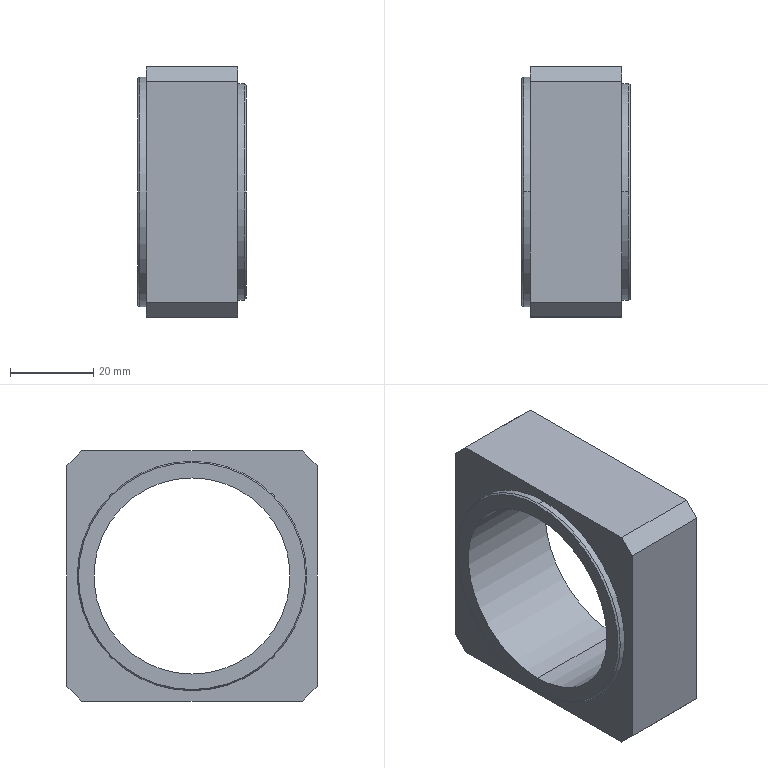Part | STEP file | _Kupplungsgehaeuse-SBG - PAS42 B | 1 solid | 22 faces | box 26 x 60 x 60 mm | volume 42515 mm3 | plane 12 | cylinder 6 | cone 4 | commonest cylinder face diameters 47 x2 52 x2 55 x2
STEP:
#1=CARTESIAN_POINT('',(26.,0.,-23.5));
#2=VERTEX_POINT('',#1);
#3=CARTESIAN_POINT('',(26.,0.,23.5));
#4=VERTEX_POINT('',#3);
#5=CARTESIAN_POINT('',(26.,0.,0.));
#6=DIRECTION('',(-1.,0.,0.));
#7=DIRECTION('',(0.,0.,1.));
#8=AXIS2_PLACEMENT_3D('',#5,#6,#7);
#9=CIRCLE('',#8,23.5);
#10=EDGE_CURVE('',#2,#4,#9,.T.);
#11=ORIENTED_EDGE('',*,*,#10,.F.);
#12=CARTESIAN_POINT('',(0.,0.,-23.5));
#13=VERTEX_POINT('',#12);
#14=CARTESIAN_POINT('',(26.,0.,-23.5));
#15=DIRECTION('',(-1.,0.,0.));
#16=VECTOR('',#15,1000.);
#17=LINE('',#14,#16);
#18=EDGE_CURVE('',#2,#13,#17,.T.);
#19=ORIENTED_EDGE('',*,*,#18,.T.);
#20=CARTESIAN_POINT('',(0.,0.,23.5));
#21=VERTEX_POINT('',#20);
#22=CARTESIAN_POINT('',(0.,0.,0.));
#23=DIRECTION('',(1.,0.,0.));
#24=DIRECTION('',(0.,0.,1.));
#25=AXIS2_PLACEMENT_3D('',#22,#23,#24);
#26=CIRCLE('',#25,23.5);
#27=EDGE_CURVE('',#21,#13,#26,.T.);
#28=ORIENTED_EDGE('',*,*,#27,.F.);
#29=CARTESIAN_POINT('',(26.,0.,23.5));
#30=DIRECTION('',(-1.,0.,0.));
#31=VECTOR('',#30,1000.);
#32=LINE('',#29,#31);
#33=EDGE_CURVE('',#4,#21,#32,.T.);
#34=ORIENTED_EDGE('',*,*,#33,.F.);
#35=EDGE_LOOP('',(#11,#19,#28,#34));
#36=FACE_OUTER_BOUND('',#35,.T.);
#37=CARTESIAN_POINT('',(26.,0.,0.));
#38=DIRECTION('',(-1.,0.,0.));
#39=DIRECTION('',(0.,0.,1.));
#40=AXIS2_PLACEMENT_3D('',#37,#38,#39);
#41=CYLINDRICAL_SURFACE('',#40,23.5);
#42=ADVANCED_FACE('',(#36),#41,.F.);
#43=CARTESIAN_POINT('',(0.,-27.211,0.));
#44=VERTEX_POINT('',#43);
#45=CARTESIAN_POINT('',(0.,27.211,0.));
#46=VERTEX_POINT('',#45);
#47=CARTESIAN_POINT('',(0.,0.,0.));
#48=DIRECTION('',(-1.,0.,0.));
#49=DIRECTION('',(0.,1.,0.));
#50=AXIS2_PLACEMENT_3D('',#47,#48,#49);
#51=CIRCLE('',#50,27.211);
#52=EDGE_CURVE('',#44,#46,#51,.T.);
#53=ORIENTED_EDGE('',*,*,#52,.F.);
#54=CARTESIAN_POINT('',(0.5,-27.5,0.));
#55=VERTEX_POINT('',#54);
#56=CARTESIAN_POINT('',(0.5,-27.5,0.));
#57=DIRECTION('',(0.866,-0.5,0.));
#58=VECTOR('',#57,1000.);
#59=LINE('',#56,#58);
#60=EDGE_CURVE('',#44,#55,#59,.T.);
#61=ORIENTED_EDGE('',*,*,#60,.T.);
#62=CARTESIAN_POINT('',(0.5,0.,27.5));
#63=VERTEX_POINT('',#62);
#64=CARTESIAN_POINT('',(0.5,0.,0.));
#65=DIRECTION('',(-1.,0.,0.));
#66=DIRECTION('',(0.,0.,-1.));
#67=AXIS2_PLACEMENT_3D('',#64,#65,#66);
#68=CIRCLE('',#67,27.5);
#69=EDGE_CURVE('',#55,#63,#68,.T.);
#70=ORIENTED_EDGE('',*,*,#69,.T.);
#71=CARTESIAN_POINT('',(0.5,27.5,0.));
#72=VERTEX_POINT('',#71);
#73=CARTESIAN_POINT('',(0.5,0.,0.));
#74=DIRECTION('',(-1.,0.,0.));
#75=DIRECTION('',(0.,0.,-1.));
#76=AXIS2_PLACEMENT_3D('',#73,#74,#75);
#77=CIRCLE('',#76,27.5);
#78=EDGE_CURVE('',#63,#72,#77,.T.);
#79=ORIENTED_EDGE('',*,*,#78,.T.);
#80=CARTESIAN_POINT('',(0.5,27.5,0.));
#81=DIRECTION('',(0.866,0.5,0.));
#82=VECTOR('',#81,1000.);
#83=LINE('',#80,#82);
#84=EDGE_CURVE('',#46,#72,#83,.T.);
#85=ORIENTED_EDGE('',*,*,#84,.F.);
#86=EDGE_LOOP('',(#53,#61,#70,#79,#85));
#87=FACE_OUTER_BOUND('',#86,.T.);
#88=CARTESIAN_POINT('',(0.5,0.,0.));
#89=DIRECTION('',(1.,0.,0.));
#90=DIRECTION('',(0.,1.,0.));
#91=AXIS2_PLACEMENT_3D('',#88,#89,#90);
#92=CONICAL_SURFACE('',#91,27.5,0.5236);
#93=ADVANCED_FACE('',(#87),#92,.T.);
#94=CARTESIAN_POINT('',(26.,25.711,0.));
#95=VERTEX_POINT('',#94);
#96=CARTESIAN_POINT('',(26.,-25.711,0.));
#97=VERTEX_POINT('',#96);
#98=CARTESIAN_POINT('',(26.,0.,0.));
#99=DIRECTION('',(1.,0.,0.));
#100=DIRECTION('',(0.,-1.,0.));
#101=AXIS2_PLACEMENT_3D('',#98,#99,#100);
#102=CIRCLE('',#101,25.711);
#103=EDGE_CURVE('',#95,#97,#102,.T.);
#104=ORIENTED_EDGE('',*,*,#103,.F.);
#105=CARTESIAN_POINT('',(25.5,26.,0.));
#106=VERTEX_POINT('',#105);
#107=CARTESIAN_POINT('',(25.5,26.,0.));
#108=DIRECTION('',(-0.866,0.5,0.));
#109=VECTOR('',#108,1000.);
#110=LINE('',#107,#109);
#111=EDGE_CURVE('',#95,#106,#110,.T.);
#112=ORIENTED_EDGE('',*,*,#111,.T.);
#113=CARTESIAN_POINT('',(25.5,0.,26.));
#114=VERTEX_POINT('',#113);
#115=CARTESIAN_POINT('',(25.5,0.,0.));
#116=DIRECTION('',(1.,0.,0.));
#117=DIRECTION('',(0.,0.,1.));
#118=AXIS2_PLACEMENT_3D('',#115,#116,#117);
#119=CIRCLE('',#118,26.);
#120=EDGE_CURVE('',#106,#114,#119,.T.);
#121=ORIENTED_EDGE('',*,*,#120,.T.);
#122=CARTESIAN_POINT('',(25.5,-26.,0.));
#123=VERTEX_POINT('',#122);
#124=CARTESIAN_POINT('',(25.5,0.,0.));
#125=DIRECTION('',(1.,0.,0.));
#126=DIRECTION('',(0.,0.,1.));
#127=AXIS2_PLACEMENT_3D('',#124,#125,#126);
#128=CIRCLE('',#127,26.);
#129=EDGE_CURVE('',#114,#123,#128,.T.);
#130=ORIENTED_EDGE('',*,*,#129,.T.);
#131=CARTESIAN_POINT('',(25.5,-26.,0.));
#132=DIRECTION('',(-0.866,-0.5,0.));
#133=VECTOR('',#132,1000.);
#134=LINE('',#131,#133);
#135=EDGE_CURVE('',#97,#123,#134,.T.);
#136=ORIENTED_EDGE('',*,*,#135,.F.);
#137=EDGE_LOOP('',(#104,#112,#121,#130,#136));
#138=FACE_OUTER_BOUND('',#137,.T.);
#139=CARTESIAN_POINT('',(25.5,0.,0.));
#140=DIRECTION('',(-1.,0.,0.));
#141=DIRECTION('',(0.,-1.,0.));
#142=AXIS2_PLACEMENT_3D('',#139,#140,#141);
#143=CONICAL_SURFACE('',#142,26.,0.5236);
#144=ADVANCED_FACE('',(#138),#143,.T.);
#145=CARTESIAN_POINT('',(2.,0.,27.5));
#146=VERTEX_POINT('',#145);
#147=CARTESIAN_POINT('',(2.,0.,-27.5));
#148=VERTEX_POINT('',#147);
#149=CARTESIAN_POINT('',(2.,0.,0.));
#150=DIRECTION('',(-1.,0.,0.));
#151=DIRECTION('',(0.,0.,1.));
#152=AXIS2_PLACEMENT_3D('',#149,#150,#151);
#153=CIRCLE('',#152,27.5);
#154=EDGE_CURVE('',#146,#148,#153,.T.);
#155=ORIENTED_EDGE('',*,*,#154,.T.);
#156=CARTESIAN_POINT('',(0.5,0.,-27.5));
#157=VERTEX_POINT('',#156);
#158=CARTESIAN_POINT('',(26.,0.,-27.5));
#159=DIRECTION('',(-1.,0.,0.));
#160=VECTOR('',#159,1000.);
#161=LINE('',#158,#160);
#162=EDGE_CURVE('',#148,#157,#161,.T.);
#163=ORIENTED_EDGE('',*,*,#162,.T.);
#164=CARTESIAN_POINT('',(0.5,0.,0.));
#165=DIRECTION('',(-1.,0.,0.));
#166=DIRECTION('',(0.,0.,-1.));
#167=AXIS2_PLACEMENT_3D('',#164,#165,#166);
#168=CIRCLE('',#167,27.5);
#169=EDGE_CURVE('',#72,#157,#168,.T.);
#170=ORIENTED_EDGE('',*,*,#169,.F.);
#171=ORIENTED_EDGE('',*,*,#78,.F.);
#172=CARTESIAN_POINT('',(26.,0.,27.5));
#173=DIRECTION('',(-1.,0.,0.));
#174=VECTOR('',#173,1000.);
#175=LINE('',#172,#174);
#176=EDGE_CURVE('',#146,#63,#175,.T.);
#177=ORIENTED_EDGE('',*,*,#176,.F.);
#178=EDGE_LOOP('',(#155,#163,#170,#171,#177));
#179=FACE_OUTER_BOUND('',#178,.T.);
#180=CARTESIAN_POINT('',(26.,0.,0.));
#181=DIRECTION('',(-1.,0.,0.));
#182=DIRECTION('',(0.,0.,1.));
#183=AXIS2_PLACEMENT_3D('',#180,#181,#182);
#184=CYLINDRICAL_SURFACE('',#183,27.5);
#185=ADVANCED_FACE('',(#179),#184,.T.);
#186=CARTESIAN_POINT('',(25.5,0.,-26.));
#187=VERTEX_POINT('',#186);
#188=CARTESIAN_POINT('',(25.5,0.,0.));
#189=DIRECTION('',(1.,0.,0.));
#190=DIRECTION('',(0.,0.,1.));
#191=AXIS2_PLACEMENT_3D('',#188,#189,#190);
#192=CIRCLE('',#191,26.);
#193=EDGE_CURVE('',#187,#106,#192,.T.);
#194=ORIENTED_EDGE('',*,*,#193,.F.);
#195=CARTESIAN_POINT('',(24.,0.,-26.));
#196=VERTEX_POINT('',#195);
#197=CARTESIAN_POINT('',(26.,0.,-26.));
#198=DIRECTION('',(-1.,0.,0.));
#199=VECTOR('',#198,1000.);
#200=LINE('',#197,#199);
#201=EDGE_CURVE('',#187,#196,#200,.T.);
#202=ORIENTED_EDGE('',*,*,#201,.T.);
#203=CARTESIAN_POINT('',(24.,0.,26.));
#204=VERTEX_POINT('',#203);
#205=CARTESIAN_POINT('',(24.,0.,0.));
#206=DIRECTION('',(1.,0.,0.));
#207=DIRECTION('',(0.,0.,1.));
#208=AXIS2_PLACEMENT_3D('',#205,#206,#207);
#209=CIRCLE('',#208,26.);
#210=EDGE_CURVE('',#196,#204,#209,.T.);
#211=ORIENTED_EDGE('',*,*,#210,.T.);
#212=CARTESIAN_POINT('',(26.,0.,26.));
#213=DIRECTION('',(-1.,0.,0.));
#214=VECTOR('',#213,1000.);
#215=LINE('',#212,#214);
#216=EDGE_CURVE('',#114,#204,#215,.T.);
#217=ORIENTED_EDGE('',*,*,#216,.F.);
#218=ORIENTED_EDGE('',*,*,#120,.F.);
#219=EDGE_LOOP('',(#194,#202,#211,#217,#218));
#220=FACE_OUTER_BOUND('',#219,.T.);
#221=CARTESIAN_POINT('',(26.,0.,0.));
#222=DIRECTION('',(-1.,0.,0.));
#223=DIRECTION('',(0.,0.,1.));
#224=AXIS2_PLACEMENT_3D('',#221,#222,#223);
#225=CYLINDRICAL_SURFACE('',#224,26.);
#226=ADVANCED_FACE('',(#220),#225,.T.);
#227=ORIENTED_EDGE('',*,*,#18,.F.);
#228=CARTESIAN_POINT('',(26.,0.,0.));
#229=DIRECTION('',(-1.,0.,0.));
#230=DIRECTION('',(0.,0.,1.));
#231=AXIS2_PLACEMENT_3D('',#228,#229,#230);
#232=CIRCLE('',#231,23.5);
#233=EDGE_CURVE('',#4,#2,#232,.T.);
#234=ORIENTED_EDGE('',*,*,#233,.F.);
#235=ORIENTED_EDGE('',*,*,#33,.T.);
#236=CARTESIAN_POINT('',(0.,0.,0.));
#237=DIRECTION('',(1.,0.,0.));
#238=DIRECTION('',(0.,0.,1.));
#239=AXIS2_PLACEMENT_3D('',#236,#237,#238);
#240=CIRCLE('',#239,23.5);
#241=EDGE_CURVE('',#13,#21,#240,.T.);
#242=ORIENTED_EDGE('',*,*,#241,.F.);
#243=EDGE_LOOP('',(#227,#234,#235,#242));
#244=FACE_OUTER_BOUND('',#243,.T.);
#245=CARTESIAN_POINT('',(26.,0.,0.));
#246=DIRECTION('',(-1.,0.,0.));
#247=DIRECTION('',(0.,0.,1.));
#248=AXIS2_PLACEMENT_3D('',#245,#246,#247);
#249=CYLINDRICAL_SURFACE('',#248,23.5);
#250=ADVANCED_FACE('',(#244),#249,.F.);
#251=CARTESIAN_POINT('',(0.,0.,0.));
#252=DIRECTION('',(-1.,0.,0.));
#253=DIRECTION('',(0.,1.,0.));
#254=AXIS2_PLACEMENT_3D('',#251,#252,#253);
#255=CIRCLE('',#254,27.211);
#256=EDGE_CURVE('',#46,#44,#255,.T.);
#257=ORIENTED_EDGE('',*,*,#256,.T.);
#258=ORIENTED_EDGE('',*,*,#52,.T.);
#259=EDGE_LOOP('',(#257,#258));
#260=FACE_OUTER_BOUND('',#259,.T.);
#261=ORIENTED_EDGE('',*,*,#27,.T.);
#262=ORIENTED_EDGE('',*,*,#241,.T.);
#263=EDGE_LOOP('',(#261,#262));
#264=FACE_BOUND('',#263,.T.);
#265=CARTESIAN_POINT('',(0.,27.211,0.));
#266=DIRECTION('',(-1.,0.,0.));
#267=DIRECTION('',(0.,0.,1.));
#268=AXIS2_PLACEMENT_3D('',#265,#266,#267);
#269=PLANE('',#268);
#270=ADVANCED_FACE('',(#260,#264),#269,.T.);
#271=ORIENTED_EDGE('',*,*,#233,.T.);
#272=ORIENTED_EDGE('',*,*,#10,.T.);
#273=EDGE_LOOP('',(#271,#272));
#274=FACE_BOUND('',#273,.T.);
#275=CARTESIAN_POINT('',(26.,0.,0.));
#276=DIRECTION('',(1.,0.,0.));
#277=DIRECTION('',(0.,-1.,0.));
#278=AXIS2_PLACEMENT_3D('',#275,#276,#277);
#279=CIRCLE('',#278,25.711);
#280=EDGE_CURVE('',#97,#95,#279,.T.);
#281=ORIENTED_EDGE('',*,*,#280,.T.);
#282=ORIENTED_EDGE('',*,*,#103,.T.);
#283=EDGE_LOOP('',(#281,#282));
#284=FACE_OUTER_BOUND('',#283,.T.);
#285=CARTESIAN_POINT('',(26.,23.5,0.));
#286=DIRECTION('',(1.,0.,0.));
#287=DIRECTION('',(0.,0.,-1.));
#288=AXIS2_PLACEMENT_3D('',#285,#286,#287);
#289=PLANE('',#288);
#290=ADVANCED_FACE('',(#274,#284),#289,.T.);
#291=ORIENTED_EDGE('',*,*,#60,.F.);
#292=ORIENTED_EDGE('',*,*,#256,.F.);
#293=ORIENTED_EDGE('',*,*,#84,.T.);
#294=ORIENTED_EDGE('',*,*,#169,.T.);
#295=CARTESIAN_POINT('',(0.5,0.,0.));
#296=DIRECTION('',(-1.,0.,0.));
#297=DIRECTION('',(0.,0.,-1.));
#298=AXIS2_PLACEMENT_3D('',#295,#296,#297);
#299=CIRCLE('',#298,27.5);
#300=EDGE_CURVE('',#157,#55,#299,.T.);
#301=ORIENTED_EDGE('',*,*,#300,.T.);
#302=EDGE_LOOP('',(#291,#292,#293,#294,#301));
#303=FACE_OUTER_BOUND('',#302,.T.);
#304=CARTESIAN_POINT('',(0.5,0.,0.));
#305=DIRECTION('',(1.,0.,0.));
#306=DIRECTION('',(0.,1.,0.));
#307=AXIS2_PLACEMENT_3D('',#304,#305,#306);
#308=CONICAL_SURFACE('',#307,27.5,0.5236);
#309=ADVANCED_FACE('',(#303),#308,.T.);
#310=ORIENTED_EDGE('',*,*,#111,.F.);
#311=ORIENTED_EDGE('',*,*,#280,.F.);
#312=ORIENTED_EDGE('',*,*,#135,.T.);
#313=CARTESIAN_POINT('',(25.5,0.,0.));
#314=DIRECTION('',(1.,0.,0.));
#315=DIRECTION('',(0.,0.,1.));
#316=AXIS2_PLACEMENT_3D('',#313,#314,#315);
#317=CIRCLE('',#316,26.);
#318=EDGE_CURVE('',#123,#187,#317,.T.);
#319=ORIENTED_EDGE('',*,*,#318,.T.);
#320=ORIENTED_EDGE('',*,*,#193,.T.);
#321=EDGE_LOOP('',(#310,#311,#312,#319,#320));
#322=FACE_OUTER_BOUND('',#321,.T.);
#323=CARTESIAN_POINT('',(25.5,0.,0.));
#324=DIRECTION('',(-1.,0.,0.));
#325=DIRECTION('',(0.,-1.,0.));
#326=AXIS2_PLACEMENT_3D('',#323,#324,#325);
#327=CONICAL_SURFACE('',#326,26.,0.5236);
#328=ADVANCED_FACE('',(#322),#327,.T.);
#329=ORIENTED_EDGE('',*,*,#162,.F.);
#330=CARTESIAN_POINT('',(2.,0.,0.));
#331=DIRECTION('',(-1.,0.,0.));
#332=DIRECTION('',(0.,0.,1.));
#333=AXIS2_PLACEMENT_3D('',#330,#331,#332);
#334=CIRCLE('',#333,27.5);
#335=EDGE_CURVE('',#148,#146,#334,.T.);
#336=ORIENTED_EDGE('',*,*,#335,.T.);
#337=ORIENTED_EDGE('',*,*,#176,.T.);
#338=ORIENTED_EDGE('',*,*,#69,.F.);
#339=ORIENTED_EDGE('',*,*,#300,.F.);
#340=EDGE_LOOP('',(#329,#336,#337,#338,#339));
#341=FACE_OUTER_BOUND('',#340,.T.);
#342=CARTESIAN_POINT('',(26.,0.,0.));
#343=DIRECTION('',(-1.,0.,0.));
#344=DIRECTION('',(0.,0.,1.));
#345=AXIS2_PLACEMENT_3D('',#342,#343,#344);
#346=CYLINDRICAL_SURFACE('',#345,27.5);
#347=ADVANCED_FACE('',(#341),#346,.T.);
#348=ORIENTED_EDGE('',*,*,#201,.F.);
#349=ORIENTED_EDGE('',*,*,#318,.F.);
#350=ORIENTED_EDGE('',*,*,#129,.F.);
#351=ORIENTED_EDGE('',*,*,#216,.T.);
#352=CARTESIAN_POINT('',(24.,0.,0.));
#353=DIRECTION('',(1.,0.,0.));
#354=DIRECTION('',(0.,0.,1.));
#355=AXIS2_PLACEMENT_3D('',#352,#353,#354);
#356=CIRCLE('',#355,26.);
#357=EDGE_CURVE('',#204,#196,#356,.T.);
#358=ORIENTED_EDGE('',*,*,#357,.T.);
#359=EDGE_LOOP('',(#348,#349,#350,#351,#358));
#360=FACE_OUTER_BOUND('',#359,.T.);
#361=CARTESIAN_POINT('',(26.,0.,0.));
#362=DIRECTION('',(-1.,0.,0.));
#363=DIRECTION('',(0.,0.,1.));
#364=AXIS2_PLACEMENT_3D('',#361,#362,#363);
#365=CYLINDRICAL_SURFACE('',#364,26.);
#366=ADVANCED_FACE('',(#360),#365,.T.);
#367=CARTESIAN_POINT('',(2.,30.,26.46));
#368=VERTEX_POINT('',#367);
#369=CARTESIAN_POINT('',(2.,26.46,30.));
#370=VERTEX_POINT('',#369);
#371=CARTESIAN_POINT('',(2.,30.,26.46));
#372=DIRECTION('',(0.,-0.7071,0.7071));
#373=VECTOR('',#372,1000.);
#374=LINE('',#371,#373);
#375=EDGE_CURVE('',#368,#370,#374,.T.);
#376=ORIENTED_EDGE('',*,*,#375,.F.);
#377=CARTESIAN_POINT('',(2.,30.,-26.46));
#378=VERTEX_POINT('',#377);
#379=CARTESIAN_POINT('',(2.,30.,0.));
#380=DIRECTION('',(0.,0.,1.));
#381=VECTOR('',#380,1000.);
#382=LINE('',#379,#381);
#383=EDGE_CURVE('',#378,#368,#382,.T.);
#384=ORIENTED_EDGE('',*,*,#383,.F.);
#385=CARTESIAN_POINT('',(2.,26.46,-30.));
#386=VERTEX_POINT('',#385);
#387=CARTESIAN_POINT('',(2.,26.46,-30.));
#388=DIRECTION('',(0.,0.7071,0.7071));
#389=VECTOR('',#388,1000.);
#390=LINE('',#387,#389);
#391=EDGE_CURVE('',#386,#378,#390,.T.);
#392=ORIENTED_EDGE('',*,*,#391,.F.);
#393=CARTESIAN_POINT('',(2.,-26.46,-30.));
#394=VERTEX_POINT('',#393);
#395=CARTESIAN_POINT('',(2.,0.,-30.));
#396=DIRECTION('',(0.,1.,0.));
#397=VECTOR('',#396,1000.);
#398=LINE('',#395,#397);
#399=EDGE_CURVE('',#394,#386,#398,.T.);
#400=ORIENTED_EDGE('',*,*,#399,.F.);
#401=CARTESIAN_POINT('',(2.,-30.,-26.46));
#402=VERTEX_POINT('',#401);
#403=CARTESIAN_POINT('',(2.,-30.,-26.46));
#404=DIRECTION('',(0.,0.7071,-0.7071));
#405=VECTOR('',#404,1000.);
#406=LINE('',#403,#405);
#407=EDGE_CURVE('',#402,#394,#406,.T.);
#408=ORIENTED_EDGE('',*,*,#407,.F.);
#409=CARTESIAN_POINT('',(2.,-30.,26.46));
#410=VERTEX_POINT('',#409);
#411=CARTESIAN_POINT('',(2.,-30.,0.));
#412=DIRECTION('',(0.,0.,-1.));
#413=VECTOR('',#412,1000.);
#414=LINE('',#411,#413);
#415=EDGE_CURVE('',#410,#402,#414,.T.);
#416=ORIENTED_EDGE('',*,*,#415,.F.);
#417=CARTESIAN_POINT('',(2.,-26.46,30.));
#418=VERTEX_POINT('',#417);
#419=CARTESIAN_POINT('',(2.,-26.46,30.));
#420=DIRECTION('',(0.,-0.7071,-0.7071));
#421=VECTOR('',#420,1000.);
#422=LINE('',#419,#421);
#423=EDGE_CURVE('',#418,#410,#422,.T.);
#424=ORIENTED_EDGE('',*,*,#423,.F.);
#425=CARTESIAN_POINT('',(2.,0.,30.));
#426=DIRECTION('',(0.,-1.,0.));
#427=VECTOR('',#426,1000.);
#428=LINE('',#425,#427);
#429=EDGE_CURVE('',#370,#418,#428,.T.);
#430=ORIENTED_EDGE('',*,*,#429,.F.);
#431=EDGE_LOOP('',(#376,#384,#392,#400,#408,#416,#424,#430));
#432=FACE_OUTER_BOUND('',#431,.T.);
#433=ORIENTED_EDGE('',*,*,#154,.F.);
#434=ORIENTED_EDGE('',*,*,#335,.F.);
#435=EDGE_LOOP('',(#433,#434));
#436=FACE_BOUND('',#435,.T.);
#437=CARTESIAN_POINT('',(2.,0.,0.));
#438=DIRECTION('',(1.,0.,0.));
#439=DIRECTION('',(0.,0.,-1.));
#440=AXIS2_PLACEMENT_3D('',#437,#438,#439);
#441=PLANE('',#440);
#442=ADVANCED_FACE('',(#432,#436),#441,.F.);
#443=CARTESIAN_POINT('',(24.,30.,-26.46));
#444=VERTEX_POINT('',#443);
#445=CARTESIAN_POINT('',(24.,30.,26.46));
#446=VERTEX_POINT('',#445);
#447=CARTESIAN_POINT('',(24.,30.,0.));
#448=DIRECTION('',(0.,0.,1.));
#449=VECTOR('',#448,1000.);
#450=LINE('',#447,#449);
#451=EDGE_CURVE('',#444,#446,#450,.T.);
#452=ORIENTED_EDGE('',*,*,#451,.T.);
#453=CARTESIAN_POINT('',(24.,26.46,30.));
#454=VERTEX_POINT('',#453);
#455=CARTESIAN_POINT('',(24.,30.,26.46));
#456=DIRECTION('',(0.,-0.7071,0.7071));
#457=VECTOR('',#456,1000.);
#458=LINE('',#455,#457);
#459=EDGE_CURVE('',#446,#454,#458,.T.);
#460=ORIENTED_EDGE('',*,*,#459,.T.);
#461=CARTESIAN_POINT('',(24.,-26.46,30.));
#462=VERTEX_POINT('',#461);
#463=CARTESIAN_POINT('',(24.,0.,30.));
#464=DIRECTION('',(0.,-1.,0.));
#465=VECTOR('',#464,1000.);
#466=LINE('',#463,#465);
#467=EDGE_CURVE('',#454,#462,#466,.T.);
#468=ORIENTED_EDGE('',*,*,#467,.T.);
#469=CARTESIAN_POINT('',(24.,-30.,26.46));
#470=VERTEX_POINT('',#469);
#471=CARTESIAN_POINT('',(24.,-26.46,30.));
#472=DIRECTION('',(0.,-0.7071,-0.7071));
#473=VECTOR('',#472,1000.);
#474=LINE('',#471,#473);
#475=EDGE_CURVE('',#462,#470,#474,.T.);
#476=ORIENTED_EDGE('',*,*,#475,.T.);
#477=CARTESIAN_POINT('',(24.,-30.,-26.46));
#478=VERTEX_POINT('',#477);
#479=CARTESIAN_POINT('',(24.,-30.,0.));
#480=DIRECTION('',(0.,0.,-1.));
#481=VECTOR('',#480,1000.);
#482=LINE('',#479,#481);
#483=EDGE_CURVE('',#470,#478,#482,.T.);
#484=ORIENTED_EDGE('',*,*,#483,.T.);
#485=CARTESIAN_POINT('',(24.,-26.46,-30.));
#486=VERTEX_POINT('',#485);
#487=CARTESIAN_POINT('',(24.,-30.,-26.46));
#488=DIRECTION('',(0.,0.7071,-0.7071));
#489=VECTOR('',#488,1000.);
#490=LINE('',#487,#489);
#491=EDGE_CURVE('',#478,#486,#490,.T.);
#492=ORIENTED_EDGE('',*,*,#491,.T.);
#493=CARTESIAN_POINT('',(24.,26.46,-30.));
#494=VERTEX_POINT('',#493);
#495=CARTESIAN_POINT('',(24.,0.,-30.));
#496=DIRECTION('',(0.,1.,0.));
#497=VECTOR('',#496,1000.);
#498=LINE('',#495,#497);
#499=EDGE_CURVE('',#486,#494,#498,.T.);
#500=ORIENTED_EDGE('',*,*,#499,.T.);
#501=CARTESIAN_POINT('',(24.,26.46,-30.));
#502=DIRECTION('',(0.,0.7071,0.7071));
#503=VECTOR('',#502,1000.);
#504=LINE('',#501,#503);
#505=EDGE_CURVE('',#494,#444,#504,.T.);
#506=ORIENTED_EDGE('',*,*,#505,.T.);
#507=EDGE_LOOP('',(#452,#460,#468,#476,#484,#492,#500,#506));
#508=FACE_OUTER_BOUND('',#507,.T.);
#509=ORIENTED_EDGE('',*,*,#357,.F.);
#510=ORIENTED_EDGE('',*,*,#210,.F.);
#511=EDGE_LOOP('',(#509,#510));
#512=FACE_BOUND('',#511,.T.);
#513=CARTESIAN_POINT('',(24.,0.,0.));
#514=DIRECTION('',(1.,0.,0.));
#515=DIRECTION('',(0.,0.,-1.));
#516=AXIS2_PLACEMENT_3D('',#513,#514,#515);
#517=PLANE('',#516);
#518=ADVANCED_FACE('',(#508,#512),#517,.T.);
#519=CARTESIAN_POINT('',(24.,-26.46,30.));
#520=DIRECTION('',(-1.,0.,0.));
#521=VECTOR('',#520,1000.);
#522=LINE('',#519,#521);
#523=EDGE_CURVE('',#462,#418,#522,.T.);
#524=ORIENTED_EDGE('',*,*,#523,.F.);
#525=ORIENTED_EDGE('',*,*,#467,.F.);
#526=CARTESIAN_POINT('',(24.,26.46,30.));
#527=DIRECTION('',(1.,0.,0.));
#528=VECTOR('',#527,1000.);
#529=LINE('',#526,#528);
#530=EDGE_CURVE('',#370,#454,#529,.T.);
#531=ORIENTED_EDGE('',*,*,#530,.F.);
#532=ORIENTED_EDGE('',*,*,#429,.T.);
#533=EDGE_LOOP('',(#524,#525,#531,#532));
#534=FACE_OUTER_BOUND('',#533,.T.);
#535=CARTESIAN_POINT('',(24.,26.46,30.));
#536=DIRECTION('',(0.,0.,-1.));
#537=DIRECTION('',(-1.,0.,0.));
#538=AXIS2_PLACEMENT_3D('',#535,#536,#537);
#539=PLANE('',#538);
#540=ADVANCED_FACE('',(#534),#539,.F.);
#541=ORIENTED_EDGE('',*,*,#530,.T.);
#542=ORIENTED_EDGE('',*,*,#459,.F.);
#543=CARTESIAN_POINT('',(24.,30.,26.46));
#544=DIRECTION('',(1.,0.,0.));
#545=VECTOR('',#544,1000.);
#546=LINE('',#543,#545);
#547=EDGE_CURVE('',#368,#446,#546,.T.);
#548=ORIENTED_EDGE('',*,*,#547,.F.);
#549=ORIENTED_EDGE('',*,*,#375,.T.);
#550=EDGE_LOOP('',(#541,#542,#548,#549));
#551=FACE_OUTER_BOUND('',#550,.T.);
#552=CARTESIAN_POINT('',(24.,30.,26.46));
#553=DIRECTION('',(0.,-0.7071,-0.7071));
#554=DIRECTION('',(0.,0.7071,-0.7071));
#555=AXIS2_PLACEMENT_3D('',#552,#553,#554);
#556=PLANE('',#555);
#557=ADVANCED_FACE('',(#551),#556,.F.);
#558=ORIENTED_EDGE('',*,*,#547,.T.);
#559=ORIENTED_EDGE('',*,*,#451,.F.);
#560=CARTESIAN_POINT('',(24.,30.,-26.46));
#561=DIRECTION('',(1.,0.,0.));
#562=VECTOR('',#561,1000.);
#563=LINE('',#560,#562);
#564=EDGE_CURVE('',#378,#444,#563,.T.);
#565=ORIENTED_EDGE('',*,*,#564,.F.);
#566=ORIENTED_EDGE('',*,*,#383,.T.);
#567=EDGE_LOOP('',(#558,#559,#565,#566));
#568=FACE_OUTER_BOUND('',#567,.T.);
#569=CARTESIAN_POINT('',(24.,30.,-26.46));
#570=DIRECTION('',(0.,-1.,0.));
#571=DIRECTION('',(0.,0.,-1.));
#572=AXIS2_PLACEMENT_3D('',#569,#570,#571);
#573=PLANE('',#572);
#574=ADVANCED_FACE('',(#568),#573,.F.);
#575=ORIENTED_EDGE('',*,*,#564,.T.);
#576=ORIENTED_EDGE('',*,*,#505,.F.);
#577=CARTESIAN_POINT('',(24.,26.46,-30.));
#578=DIRECTION('',(1.,0.,0.));
#579=VECTOR('',#578,1000.);
#580=LINE('',#577,#579);
#581=EDGE_CURVE('',#386,#494,#580,.T.);
#582=ORIENTED_EDGE('',*,*,#581,.F.);
#583=ORIENTED_EDGE('',*,*,#391,.T.);
#584=EDGE_LOOP('',(#575,#576,#582,#583));
#585=FACE_OUTER_BOUND('',#584,.T.);
#586=CARTESIAN_POINT('',(24.,26.46,-30.));
#587=DIRECTION('',(0.,-0.7071,0.7071));
#588=DIRECTION('',(0.,-0.7071,-0.7071));
#589=AXIS2_PLACEMENT_3D('',#586,#587,#588);
#590=PLANE('',#589);
#591=ADVANCED_FACE('',(#585),#590,.F.);
#592=ORIENTED_EDGE('',*,*,#581,.T.);
#593=ORIENTED_EDGE('',*,*,#499,.F.);
#594=CARTESIAN_POINT('',(24.,-26.46,-30.));
#595=DIRECTION('',(1.,0.,0.));
#596=VECTOR('',#595,1000.);
#597=LINE('',#594,#596);
#598=EDGE_CURVE('',#394,#486,#597,.T.);
#599=ORIENTED_EDGE('',*,*,#598,.F.);
#600=ORIENTED_EDGE('',*,*,#399,.T.);
#601=EDGE_LOOP('',(#592,#593,#599,#600));
#602=FACE_OUTER_BOUND('',#601,.T.);
#603=CARTESIAN_POINT('',(24.,-26.46,-30.));
#604=DIRECTION('',(0.,0.,1.));
#605=DIRECTION('',(1.,0.,0.));
#606=AXIS2_PLACEMENT_3D('',#603,#604,#605);
#607=PLANE('',#606);
#608=ADVANCED_FACE('',(#602),#607,.F.);
#609=ORIENTED_EDGE('',*,*,#598,.T.);
#610=ORIENTED_EDGE('',*,*,#491,.F.);
#611=CARTESIAN_POINT('',(24.,-30.,-26.46));
#612=DIRECTION('',(1.,0.,0.));
#613=VECTOR('',#612,1000.);
#614=LINE('',#611,#613);
#615=EDGE_CURVE('',#402,#478,#614,.T.);
#616=ORIENTED_EDGE('',*,*,#615,.F.);
#617=ORIENTED_EDGE('',*,*,#407,.T.);
#618=EDGE_LOOP('',(#609,#610,#616,#617));
#619=FACE_OUTER_BOUND('',#618,.T.);
#620=CARTESIAN_POINT('',(24.,-30.,-26.46));
#621=DIRECTION('',(0.,0.7071,0.7071));
#622=DIRECTION('',(0.,-0.7071,0.7071));
#623=AXIS2_PLACEMENT_3D('',#620,#621,#622);
#624=PLANE('',#623);
#625=ADVANCED_FACE('',(#619),#624,.F.);
#626=ORIENTED_EDGE('',*,*,#615,.T.);
#627=ORIENTED_EDGE('',*,*,#483,.F.);
#628=CARTESIAN_POINT('',(24.,-30.,26.46));
#629=DIRECTION('',(1.,0.,0.));
#630=VECTOR('',#629,1000.);
#631=LINE('',#628,#630);
#632=EDGE_CURVE('',#410,#470,#631,.T.);
#633=ORIENTED_EDGE('',*,*,#632,.F.);
#634=ORIENTED_EDGE('',*,*,#415,.T.);
#635=EDGE_LOOP('',(#626,#627,#633,#634));
#636=FACE_OUTER_BOUND('',#635,.T.);
#637=CARTESIAN_POINT('',(24.,-30.,26.46));
#638=DIRECTION('',(0.,1.,0.));
#639=DIRECTION('',(0.,0.,1.));
#640=AXIS2_PLACEMENT_3D('',#637,#638,#639);
#641=PLANE('',#640);
#642=ADVANCED_FACE('',(#636),#641,.F.);
#643=ORIENTED_EDGE('',*,*,#632,.T.);
#644=ORIENTED_EDGE('',*,*,#475,.F.);
#645=ORIENTED_EDGE('',*,*,#523,.T.);
#646=ORIENTED_EDGE('',*,*,#423,.T.);
#647=EDGE_LOOP('',(#643,#644,#645,#646));
#648=FACE_OUTER_BOUND('',#647,.T.);
#649=CARTESIAN_POINT('',(24.,-26.46,30.));
#650=DIRECTION('',(0.,0.7071,-0.7071));
#651=DIRECTION('',(0.,0.7071,0.7071));
#652=AXIS2_PLACEMENT_3D('',#649,#650,#651);
#653=PLANE('',#652);
#654=ADVANCED_FACE('',(#648),#653,.F.);
#655=CLOSED_SHELL('',(#42,#93,#144,#185,#226,#250,#270,#290,#309,#328,#347,#366,#442,#518,#540,#557,#574,#591,#608,#625,#642,#654));
#656=MANIFOLD_SOLID_BREP('',#655);
#657=CARTESIAN_POINT('',(0.,0.,0.));
#658=DIRECTION('',(0.,0.,1.));
#659=DIRECTION('',(1.,0.,0.));
#660=AXIS2_PLACEMENT_3D('',#657,#658,#659);
#661=(LENGTH_UNIT()NAMED_UNIT(*)SI_UNIT(.MILLI.,.METRE.));
#662=UNCERTAINTY_MEASURE_WITH_UNIT(LENGTH_MEASURE(0.00001),#661,'','');
#663=(NAMED_UNIT(*)PLANE_ANGLE_UNIT()SI_UNIT($,.RADIAN.));
#664=(NAMED_UNIT(*)SI_UNIT($,.STERADIAN.)SOLID_ANGLE_UNIT());
#665=(GEOMETRIC_REPRESENTATION_CONTEXT(3)GLOBAL_UNCERTAINTY_ASSIGNED_CONTEXT((#662))GLOBAL_UNIT_ASSIGNED_CONTEXT((#661,#663,#664))REPRESENTATION_CONTEXT('',''));
#666=ADVANCED_BREP_SHAPE_REPRESENTATION('',(#656,#660),#665);